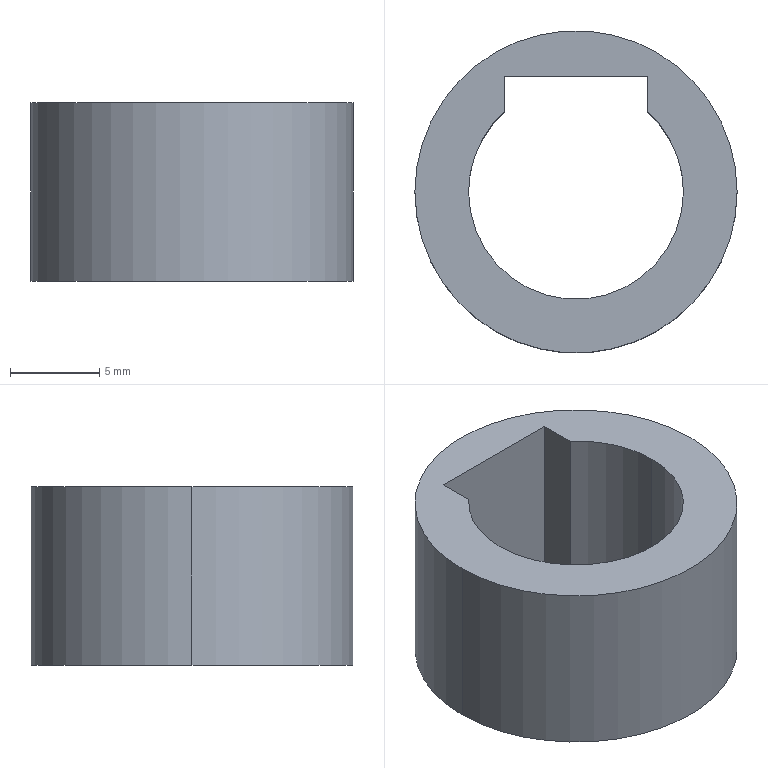Part | SolidWorks | features Extrusion 1 | 1 solid | 10 faces | box 18 x 18 x 10 mm | volume 1338 mm3 | cylinder 5 | plane 5 | commonest cylinder face diameters 12 x3 18 x2
STEP:
#1=CARTESIAN_POINT('',(-6.275,-0.1517,10.));
#2=VERTEX_POINT('',#1);
#3=CARTESIAN_POINT('',(5.725,-0.1517,10.));
#4=VERTEX_POINT('',#3);
#5=CARTESIAN_POINT('',(-0.2749,-0.1517,10.));
#6=DIRECTION('',(0.,0.,1.));
#7=DIRECTION('',(1.,0.,0.));
#8=AXIS2_PLACEMENT_3D('',#5,#6,#7);
#9=CIRCLE('',#8,6.);
#10=EDGE_CURVE('',#2,#4,#9,.T.);
#11=ORIENTED_EDGE('',*,*,#10,.T.);
#12=CARTESIAN_POINT('',(5.725,-0.1517,0.));
#13=VERTEX_POINT('',#12);
#14=CARTESIAN_POINT('',(5.725,-0.1517,10.));
#15=DIRECTION('',(0.,0.,-1.));
#16=VECTOR('',#15,1000.);
#17=LINE('',#14,#16);
#18=EDGE_CURVE('',#4,#13,#17,.T.);
#19=ORIENTED_EDGE('',*,*,#18,.T.);
#20=CARTESIAN_POINT('',(-6.275,-0.1517,0.));
#21=VERTEX_POINT('',#20);
#22=CARTESIAN_POINT('',(-0.2749,-0.1517,0.));
#23=DIRECTION('',(0.,0.,1.));
#24=DIRECTION('',(1.,0.,0.));
#25=AXIS2_PLACEMENT_3D('',#22,#23,#24);
#26=CIRCLE('',#25,6.);
#27=EDGE_CURVE('',#21,#13,#26,.T.);
#28=ORIENTED_EDGE('',*,*,#27,.F.);
#29=CARTESIAN_POINT('',(-6.275,-0.1517,10.));
#30=DIRECTION('',(0.,0.,-1.));
#31=VECTOR('',#30,1000.);
#32=LINE('',#29,#31);
#33=EDGE_CURVE('',#2,#21,#32,.T.);
#34=ORIENTED_EDGE('',*,*,#33,.F.);
#35=EDGE_LOOP('',(#11,#19,#28,#34));
#36=FACE_OUTER_BOUND('',#35,.T.);
#37=CARTESIAN_POINT('',(-0.2749,-0.1517,10.));
#38=DIRECTION('',(0.,0.,-1.));
#39=DIRECTION('',(-1.,0.,0.));
#40=AXIS2_PLACEMENT_3D('',#37,#38,#39);
#41=CYLINDRICAL_SURFACE('',#40,6.);
#42=ADVANCED_FACE('',(#36),#41,.F.);
#43=CARTESIAN_POINT('',(-4.275,4.32,10.));
#44=VERTEX_POINT('',#43);
#45=CARTESIAN_POINT('',(-0.2749,-0.1517,10.));
#46=DIRECTION('',(0.,0.,1.));
#47=DIRECTION('',(1.,0.,0.));
#48=AXIS2_PLACEMENT_3D('',#45,#46,#47);
#49=CIRCLE('',#48,6.);
#50=EDGE_CURVE('',#44,#2,#49,.T.);
#51=ORIENTED_EDGE('',*,*,#50,.T.);
#52=ORIENTED_EDGE('',*,*,#33,.T.);
#53=CARTESIAN_POINT('',(-4.275,4.32,0.));
#54=VERTEX_POINT('',#53);
#55=CARTESIAN_POINT('',(-0.2749,-0.1517,0.));
#56=DIRECTION('',(0.,0.,1.));
#57=DIRECTION('',(1.,0.,0.));
#58=AXIS2_PLACEMENT_3D('',#55,#56,#57);
#59=CIRCLE('',#58,6.);
#60=EDGE_CURVE('',#54,#21,#59,.T.);
#61=ORIENTED_EDGE('',*,*,#60,.F.);
#62=CARTESIAN_POINT('',(-4.275,4.32,10.));
#63=DIRECTION('',(0.,0.,-1.));
#64=VECTOR('',#63,1000.);
#65=LINE('',#62,#64);
#66=EDGE_CURVE('',#44,#54,#65,.T.);
#67=ORIENTED_EDGE('',*,*,#66,.F.);
#68=EDGE_LOOP('',(#51,#52,#61,#67));
#69=FACE_OUTER_BOUND('',#68,.T.);
#70=CARTESIAN_POINT('',(-0.2749,-0.1517,10.));
#71=DIRECTION('',(0.,0.,-1.));
#72=DIRECTION('',(-1.,0.,0.));
#73=AXIS2_PLACEMENT_3D('',#70,#71,#72);
#74=CYLINDRICAL_SURFACE('',#73,6.);
#75=ADVANCED_FACE('',(#69),#74,.F.);
#76=CARTESIAN_POINT('',(8.725,-0.1517,10.));
#77=VERTEX_POINT('',#76);
#78=CARTESIAN_POINT('',(-9.275,-0.1517,10.));
#79=VERTEX_POINT('',#78);
#80=CARTESIAN_POINT('',(-0.2749,-0.1517,10.));
#81=DIRECTION('',(0.,0.,1.));
#82=DIRECTION('',(1.,0.,0.));
#83=AXIS2_PLACEMENT_3D('',#80,#81,#82);
#84=CIRCLE('',#83,9.);
#85=EDGE_CURVE('',#77,#79,#84,.T.);
#86=ORIENTED_EDGE('',*,*,#85,.F.);
#87=CARTESIAN_POINT('',(8.725,-0.1517,0.));
#88=VERTEX_POINT('',#87);
#89=CARTESIAN_POINT('',(8.725,-0.1517,10.));
#90=DIRECTION('',(0.,0.,-1.));
#91=VECTOR('',#90,1000.);
#92=LINE('',#89,#91);
#93=EDGE_CURVE('',#77,#88,#92,.T.);
#94=ORIENTED_EDGE('',*,*,#93,.T.);
#95=CARTESIAN_POINT('',(-9.275,-0.1517,0.));
#96=VERTEX_POINT('',#95);
#97=CARTESIAN_POINT('',(-0.2749,-0.1517,0.));
#98=DIRECTION('',(0.,0.,1.));
#99=DIRECTION('',(1.,0.,0.));
#100=AXIS2_PLACEMENT_3D('',#97,#98,#99);
#101=CIRCLE('',#100,9.);
#102=EDGE_CURVE('',#88,#96,#101,.T.);
#103=ORIENTED_EDGE('',*,*,#102,.T.);
#104=CARTESIAN_POINT('',(-9.275,-0.1517,10.));
#105=DIRECTION('',(0.,0.,-1.));
#106=VECTOR('',#105,1000.);
#107=LINE('',#104,#106);
#108=EDGE_CURVE('',#79,#96,#107,.T.);
#109=ORIENTED_EDGE('',*,*,#108,.F.);
#110=EDGE_LOOP('',(#86,#94,#103,#109));
#111=FACE_OUTER_BOUND('',#110,.T.);
#112=CARTESIAN_POINT('',(-0.2749,-0.1517,10.));
#113=DIRECTION('',(0.,0.,-1.));
#114=DIRECTION('',(-1.,0.,0.));
#115=AXIS2_PLACEMENT_3D('',#112,#113,#114);
#116=CYLINDRICAL_SURFACE('',#115,9.);
#117=ADVANCED_FACE('',(#111),#116,.T.);
#118=CARTESIAN_POINT('',(-0.2749,-0.1517,10.));
#119=DIRECTION('',(0.,0.,1.));
#120=DIRECTION('',(1.,0.,0.));
#121=AXIS2_PLACEMENT_3D('',#118,#119,#120);
#122=CIRCLE('',#121,9.);
#123=EDGE_CURVE('',#79,#77,#122,.T.);
#124=ORIENTED_EDGE('',*,*,#123,.T.);
#125=ORIENTED_EDGE('',*,*,#85,.T.);
#126=EDGE_LOOP('',(#124,#125));
#127=FACE_OUTER_BOUND('',#126,.T.);
#128=ORIENTED_EDGE('',*,*,#50,.F.);
#129=CARTESIAN_POINT('',(-4.275,6.32,10.));
#130=VERTEX_POINT('',#129);
#131=CARTESIAN_POINT('',(-4.275,6.32,10.));
#132=DIRECTION('',(0.,-1.,0.));
#133=VECTOR('',#132,1000.);
#134=LINE('',#131,#133);
#135=EDGE_CURVE('',#130,#44,#134,.T.);
#136=ORIENTED_EDGE('',*,*,#135,.F.);
#137=CARTESIAN_POINT('',(3.725,6.32,10.));
#138=VERTEX_POINT('',#137);
#139=CARTESIAN_POINT('',(-4.275,6.32,10.));
#140=DIRECTION('',(-1.,0.,0.));
#141=VECTOR('',#140,1000.);
#142=LINE('',#139,#141);
#143=EDGE_CURVE('',#138,#130,#142,.T.);
#144=ORIENTED_EDGE('',*,*,#143,.F.);
#145=CARTESIAN_POINT('',(3.725,4.32,10.));
#146=VERTEX_POINT('',#145);
#147=CARTESIAN_POINT('',(3.725,6.32,10.));
#148=DIRECTION('',(0.,1.,0.));
#149=VECTOR('',#148,1000.);
#150=LINE('',#147,#149);
#151=EDGE_CURVE('',#146,#138,#150,.T.);
#152=ORIENTED_EDGE('',*,*,#151,.F.);
#153=CARTESIAN_POINT('',(-0.2749,-0.1517,10.));
#154=DIRECTION('',(0.,0.,1.));
#155=DIRECTION('',(1.,0.,0.));
#156=AXIS2_PLACEMENT_3D('',#153,#154,#155);
#157=CIRCLE('',#156,6.);
#158=EDGE_CURVE('',#4,#146,#157,.T.);
#159=ORIENTED_EDGE('',*,*,#158,.F.);
#160=ORIENTED_EDGE('',*,*,#10,.F.);
#161=EDGE_LOOP('',(#128,#136,#144,#152,#159,#160));
#162=FACE_BOUND('',#161,.T.);
#163=CARTESIAN_POINT('',(-0.2749,-0.1517,10.));
#164=DIRECTION('',(0.,0.,1.));
#165=DIRECTION('',(1.,0.,0.));
#166=AXIS2_PLACEMENT_3D('',#163,#164,#165);
#167=PLANE('',#166);
#168=ADVANCED_FACE('',(#127,#162),#167,.T.);
#169=CARTESIAN_POINT('',(-0.2749,-0.1517,0.));
#170=DIRECTION('',(0.,0.,1.));
#171=DIRECTION('',(1.,0.,0.));
#172=AXIS2_PLACEMENT_3D('',#169,#170,#171);
#173=CIRCLE('',#172,9.);
#174=EDGE_CURVE('',#96,#88,#173,.T.);
#175=ORIENTED_EDGE('',*,*,#174,.F.);
#176=ORIENTED_EDGE('',*,*,#102,.F.);
#177=EDGE_LOOP('',(#175,#176));
#178=FACE_OUTER_BOUND('',#177,.T.);
#179=CARTESIAN_POINT('',(-4.275,6.32,0.));
#180=VERTEX_POINT('',#179);
#181=CARTESIAN_POINT('',(-4.275,6.32,0.));
#182=DIRECTION('',(0.,-1.,0.));
#183=VECTOR('',#182,1000.);
#184=LINE('',#181,#183);
#185=EDGE_CURVE('',#180,#54,#184,.T.);
#186=ORIENTED_EDGE('',*,*,#185,.T.);
#187=ORIENTED_EDGE('',*,*,#60,.T.);
#188=ORIENTED_EDGE('',*,*,#27,.T.);
#189=CARTESIAN_POINT('',(3.725,4.32,0.));
#190=VERTEX_POINT('',#189);
#191=CARTESIAN_POINT('',(-0.2749,-0.1517,0.));
#192=DIRECTION('',(0.,0.,1.));
#193=DIRECTION('',(1.,0.,0.));
#194=AXIS2_PLACEMENT_3D('',#191,#192,#193);
#195=CIRCLE('',#194,6.);
#196=EDGE_CURVE('',#13,#190,#195,.T.);
#197=ORIENTED_EDGE('',*,*,#196,.T.);
#198=CARTESIAN_POINT('',(3.725,6.32,0.));
#199=VERTEX_POINT('',#198);
#200=CARTESIAN_POINT('',(3.725,6.32,0.));
#201=DIRECTION('',(0.,1.,0.));
#202=VECTOR('',#201,1000.);
#203=LINE('',#200,#202);
#204=EDGE_CURVE('',#190,#199,#203,.T.);
#205=ORIENTED_EDGE('',*,*,#204,.T.);
#206=CARTESIAN_POINT('',(-4.275,6.32,0.));
#207=DIRECTION('',(-1.,0.,0.));
#208=VECTOR('',#207,1000.);
#209=LINE('',#206,#208);
#210=EDGE_CURVE('',#199,#180,#209,.T.);
#211=ORIENTED_EDGE('',*,*,#210,.T.);
#212=EDGE_LOOP('',(#186,#187,#188,#197,#205,#211));
#213=FACE_BOUND('',#212,.T.);
#214=CARTESIAN_POINT('',(-0.2749,-0.1517,0.));
#215=DIRECTION('',(0.,0.,1.));
#216=DIRECTION('',(1.,0.,0.));
#217=AXIS2_PLACEMENT_3D('',#214,#215,#216);
#218=PLANE('',#217);
#219=ADVANCED_FACE('',(#178,#213),#218,.F.);
#220=ORIENTED_EDGE('',*,*,#93,.F.);
#221=ORIENTED_EDGE('',*,*,#123,.F.);
#222=ORIENTED_EDGE('',*,*,#108,.T.);
#223=ORIENTED_EDGE('',*,*,#174,.T.);
#224=EDGE_LOOP('',(#220,#221,#222,#223));
#225=FACE_OUTER_BOUND('',#224,.T.);
#226=CARTESIAN_POINT('',(-0.2749,-0.1517,10.));
#227=DIRECTION('',(0.,0.,-1.));
#228=DIRECTION('',(-1.,0.,0.));
#229=AXIS2_PLACEMENT_3D('',#226,#227,#228);
#230=CYLINDRICAL_SURFACE('',#229,9.);
#231=ADVANCED_FACE('',(#225),#230,.T.);
#232=ORIENTED_EDGE('',*,*,#185,.F.);
#233=CARTESIAN_POINT('',(-4.275,6.32,10.));
#234=DIRECTION('',(0.,0.,-1.));
#235=VECTOR('',#234,1000.);
#236=LINE('',#233,#235);
#237=EDGE_CURVE('',#130,#180,#236,.T.);
#238=ORIENTED_EDGE('',*,*,#237,.F.);
#239=ORIENTED_EDGE('',*,*,#135,.T.);
#240=ORIENTED_EDGE('',*,*,#66,.T.);
#241=EDGE_LOOP('',(#232,#238,#239,#240));
#242=FACE_OUTER_BOUND('',#241,.T.);
#243=CARTESIAN_POINT('',(-4.275,6.32,10.));
#244=DIRECTION('',(1.,0.,0.));
#245=DIRECTION('',(0.,0.,-1.));
#246=AXIS2_PLACEMENT_3D('',#243,#244,#245);
#247=PLANE('',#246);
#248=ADVANCED_FACE('',(#242),#247,.T.);
#249=ORIENTED_EDGE('',*,*,#18,.F.);
#250=ORIENTED_EDGE('',*,*,#158,.T.);
#251=CARTESIAN_POINT('',(3.725,4.32,10.));
#252=DIRECTION('',(0.,0.,-1.));
#253=VECTOR('',#252,1000.);
#254=LINE('',#251,#253);
#255=EDGE_CURVE('',#146,#190,#254,.T.);
#256=ORIENTED_EDGE('',*,*,#255,.T.);
#257=ORIENTED_EDGE('',*,*,#196,.F.);
#258=EDGE_LOOP('',(#249,#250,#256,#257));
#259=FACE_OUTER_BOUND('',#258,.T.);
#260=CARTESIAN_POINT('',(-0.2749,-0.1517,10.));
#261=DIRECTION('',(0.,0.,-1.));
#262=DIRECTION('',(-1.,0.,0.));
#263=AXIS2_PLACEMENT_3D('',#260,#261,#262);
#264=CYLINDRICAL_SURFACE('',#263,6.);
#265=ADVANCED_FACE('',(#259),#264,.F.);
#266=ORIENTED_EDGE('',*,*,#204,.F.);
#267=ORIENTED_EDGE('',*,*,#255,.F.);
#268=ORIENTED_EDGE('',*,*,#151,.T.);
#269=CARTESIAN_POINT('',(3.725,6.32,10.));
#270=DIRECTION('',(0.,0.,-1.));
#271=VECTOR('',#270,1000.);
#272=LINE('',#269,#271);
#273=EDGE_CURVE('',#138,#199,#272,.T.);
#274=ORIENTED_EDGE('',*,*,#273,.T.);
#275=EDGE_LOOP('',(#266,#267,#268,#274));
#276=FACE_OUTER_BOUND('',#275,.T.);
#277=CARTESIAN_POINT('',(3.725,6.32,10.));
#278=DIRECTION('',(-1.,0.,0.));
#279=DIRECTION('',(0.,0.,1.));
#280=AXIS2_PLACEMENT_3D('',#277,#278,#279);
#281=PLANE('',#280);
#282=ADVANCED_FACE('',(#276),#281,.T.);
#283=ORIENTED_EDGE('',*,*,#210,.F.);
#284=ORIENTED_EDGE('',*,*,#273,.F.);
#285=ORIENTED_EDGE('',*,*,#143,.T.);
#286=ORIENTED_EDGE('',*,*,#237,.T.);
#287=EDGE_LOOP('',(#283,#284,#285,#286));
#288=FACE_OUTER_BOUND('',#287,.T.);
#289=CARTESIAN_POINT('',(-4.275,6.32,10.));
#290=DIRECTION('',(0.,-1.,0.));
#291=DIRECTION('',(0.,0.,-1.));
#292=AXIS2_PLACEMENT_3D('',#289,#290,#291);
#293=PLANE('',#292);
#294=ADVANCED_FACE('',(#288),#293,.T.);
#295=CLOSED_SHELL('',(#42,#75,#117,#168,#219,#231,#248,#265,#282,#294));
#296=MANIFOLD_SOLID_BREP('',#295);
#297=CARTESIAN_POINT('',(0.,0.,0.));
#298=DIRECTION('',(0.,0.,1.));
#299=DIRECTION('',(1.,0.,0.));
#300=AXIS2_PLACEMENT_3D('',#297,#298,#299);
#301=(LENGTH_UNIT()NAMED_UNIT(*)SI_UNIT(.MILLI.,.METRE.));
#302=UNCERTAINTY_MEASURE_WITH_UNIT(LENGTH_MEASURE(0.00001),#301,'','');
#303=(NAMED_UNIT(*)PLANE_ANGLE_UNIT()SI_UNIT($,.RADIAN.));
#304=(NAMED_UNIT(*)SI_UNIT($,.STERADIAN.)SOLID_ANGLE_UNIT());
#305=(GEOMETRIC_REPRESENTATION_CONTEXT(3)GLOBAL_UNCERTAINTY_ASSIGNED_CONTEXT((#302))GLOBAL_UNIT_ASSIGNED_CONTEXT((#301,#303,#304))REPRESENTATION_CONTEXT('',''));
#306=ADVANCED_BREP_SHAPE_REPRESENTATION('',(#296,#300),#305);